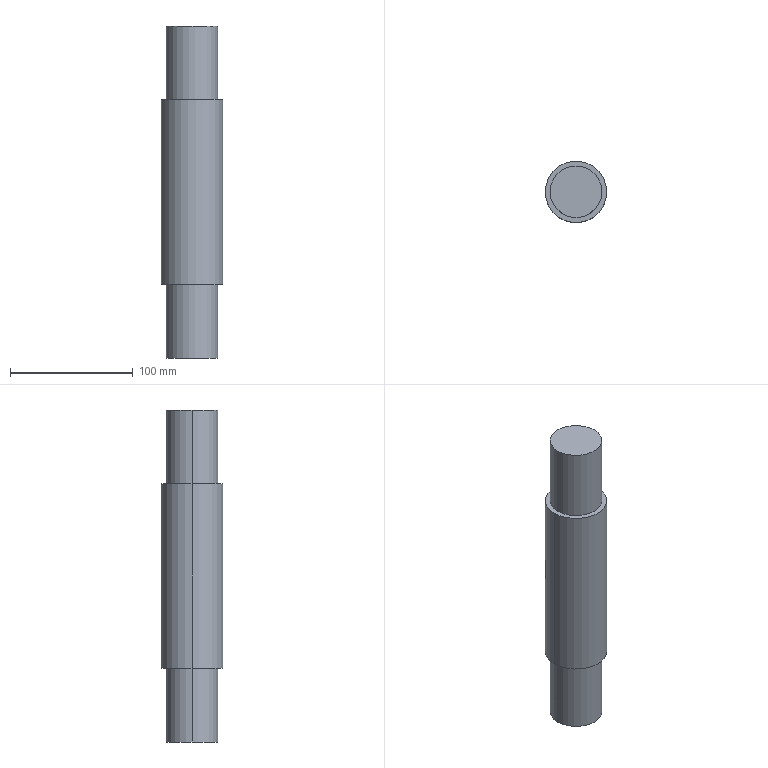Part | SolidWorks | features Extrusion 1, ICE 1, MirrorPattern 1 | 1 solid | 10 faces | box 50 x 50 x 270 mm | volume 460777 mm3 | cylinder 6 | plane 4 | commonest cylinder face diameters 42 x4 50 x2
STEP:
#1=CARTESIAN_POINT('',(21.,0.,-135.));
#2=VERTEX_POINT('',#1);
#3=CARTESIAN_POINT('',(-21.,0.,-135.));
#4=VERTEX_POINT('',#3);
#5=CARTESIAN_POINT('',(0.,0.,-135.));
#6=DIRECTION('',(0.,0.,1.));
#7=DIRECTION('',(1.,0.,0.));
#8=AXIS2_PLACEMENT_3D('',#5,#6,#7);
#9=CIRCLE('',#8,21.);
#10=EDGE_CURVE('',#2,#4,#9,.T.);
#11=ORIENTED_EDGE('',*,*,#10,.T.);
#12=CARTESIAN_POINT('',(-21.,0.,-75.));
#13=VERTEX_POINT('',#12);
#14=CARTESIAN_POINT('',(-21.,0.,-135.));
#15=DIRECTION('',(0.,0.,1.));
#16=VECTOR('',#15,1000.);
#17=LINE('',#14,#16);
#18=EDGE_CURVE('',#4,#13,#17,.T.);
#19=ORIENTED_EDGE('',*,*,#18,.T.);
#20=CARTESIAN_POINT('',(21.,0.,-75.));
#21=VERTEX_POINT('',#20);
#22=CARTESIAN_POINT('',(0.,0.,-75.));
#23=DIRECTION('',(0.,0.,1.));
#24=DIRECTION('',(1.,0.,0.));
#25=AXIS2_PLACEMENT_3D('',#22,#23,#24);
#26=CIRCLE('',#25,21.);
#27=EDGE_CURVE('',#21,#13,#26,.T.);
#28=ORIENTED_EDGE('',*,*,#27,.F.);
#29=CARTESIAN_POINT('',(21.,0.,-135.));
#30=DIRECTION('',(0.,0.,1.));
#31=VECTOR('',#30,1000.);
#32=LINE('',#29,#31);
#33=EDGE_CURVE('',#2,#21,#32,.T.);
#34=ORIENTED_EDGE('',*,*,#33,.F.);
#35=EDGE_LOOP('',(#11,#19,#28,#34));
#36=FACE_OUTER_BOUND('',#35,.T.);
#37=CARTESIAN_POINT('',(0.,0.,-135.));
#38=DIRECTION('',(0.,0.,1.));
#39=DIRECTION('',(1.,0.,0.));
#40=AXIS2_PLACEMENT_3D('',#37,#38,#39);
#41=CYLINDRICAL_SURFACE('',#40,21.);
#42=ADVANCED_FACE('',(#36),#41,.T.);
#43=CARTESIAN_POINT('',(21.,0.,135.));
#44=VERTEX_POINT('',#43);
#45=CARTESIAN_POINT('',(-21.,0.,135.));
#46=VERTEX_POINT('',#45);
#47=CARTESIAN_POINT('',(0.,0.,135.));
#48=DIRECTION('',(0.,0.,1.));
#49=DIRECTION('',(1.,0.,0.));
#50=AXIS2_PLACEMENT_3D('',#47,#48,#49);
#51=CIRCLE('',#50,21.);
#52=EDGE_CURVE('',#44,#46,#51,.T.);
#53=ORIENTED_EDGE('',*,*,#52,.F.);
#54=CARTESIAN_POINT('',(21.,0.,75.));
#55=VERTEX_POINT('',#54);
#56=CARTESIAN_POINT('',(21.,0.,135.));
#57=DIRECTION('',(0.,0.,-1.));
#58=VECTOR('',#57,1000.);
#59=LINE('',#56,#58);
#60=EDGE_CURVE('',#44,#55,#59,.T.);
#61=ORIENTED_EDGE('',*,*,#60,.T.);
#62=CARTESIAN_POINT('',(-21.,0.,75.));
#63=VERTEX_POINT('',#62);
#64=CARTESIAN_POINT('',(0.,0.,75.));
#65=DIRECTION('',(0.,0.,1.));
#66=DIRECTION('',(1.,0.,0.));
#67=AXIS2_PLACEMENT_3D('',#64,#65,#66);
#68=CIRCLE('',#67,21.);
#69=EDGE_CURVE('',#55,#63,#68,.T.);
#70=ORIENTED_EDGE('',*,*,#69,.T.);
#71=CARTESIAN_POINT('',(-21.,0.,135.));
#72=DIRECTION('',(0.,0.,-1.));
#73=VECTOR('',#72,1000.);
#74=LINE('',#71,#73);
#75=EDGE_CURVE('',#46,#63,#74,.T.);
#76=ORIENTED_EDGE('',*,*,#75,.F.);
#77=EDGE_LOOP('',(#53,#61,#70,#76));
#78=FACE_OUTER_BOUND('',#77,.T.);
#79=CARTESIAN_POINT('',(0.,0.,135.));
#80=DIRECTION('',(0.,0.,-1.));
#81=DIRECTION('',(-1.,0.,0.));
#82=AXIS2_PLACEMENT_3D('',#79,#80,#81);
#83=CYLINDRICAL_SURFACE('',#82,21.);
#84=ADVANCED_FACE('',(#78),#83,.T.);
#85=CARTESIAN_POINT('',(25.,0.,75.));
#86=VERTEX_POINT('',#85);
#87=CARTESIAN_POINT('',(-25.,0.,75.));
#88=VERTEX_POINT('',#87);
#89=CARTESIAN_POINT('',(0.,0.,75.));
#90=DIRECTION('',(0.,0.,1.));
#91=DIRECTION('',(1.,0.,0.));
#92=AXIS2_PLACEMENT_3D('',#89,#90,#91);
#93=CIRCLE('',#92,25.);
#94=EDGE_CURVE('',#86,#88,#93,.T.);
#95=ORIENTED_EDGE('',*,*,#94,.F.);
#96=CARTESIAN_POINT('',(25.,0.,-75.));
#97=VERTEX_POINT('',#96);
#98=CARTESIAN_POINT('',(25.,0.,75.));
#99=DIRECTION('',(0.,0.,-1.));
#100=VECTOR('',#99,1000.);
#101=LINE('',#98,#100);
#102=EDGE_CURVE('',#86,#97,#101,.T.);
#103=ORIENTED_EDGE('',*,*,#102,.T.);
#104=CARTESIAN_POINT('',(-25.,0.,-75.));
#105=VERTEX_POINT('',#104);
#106=CARTESIAN_POINT('',(0.,0.,-75.));
#107=DIRECTION('',(0.,0.,1.));
#108=DIRECTION('',(1.,0.,0.));
#109=AXIS2_PLACEMENT_3D('',#106,#107,#108);
#110=CIRCLE('',#109,25.);
#111=EDGE_CURVE('',#97,#105,#110,.T.);
#112=ORIENTED_EDGE('',*,*,#111,.T.);
#113=CARTESIAN_POINT('',(-25.,0.,75.));
#114=DIRECTION('',(0.,0.,-1.));
#115=VECTOR('',#114,1000.);
#116=LINE('',#113,#115);
#117=EDGE_CURVE('',#88,#105,#116,.T.);
#118=ORIENTED_EDGE('',*,*,#117,.F.);
#119=EDGE_LOOP('',(#95,#103,#112,#118));
#120=FACE_OUTER_BOUND('',#119,.T.);
#121=CARTESIAN_POINT('',(0.,0.,75.));
#122=DIRECTION('',(0.,0.,-1.));
#123=DIRECTION('',(-1.,0.,0.));
#124=AXIS2_PLACEMENT_3D('',#121,#122,#123);
#125=CYLINDRICAL_SURFACE('',#124,25.);
#126=ADVANCED_FACE('',(#120),#125,.T.);
#127=ORIENTED_EDGE('',*,*,#102,.F.);
#128=CARTESIAN_POINT('',(0.,0.,75.));
#129=DIRECTION('',(0.,0.,1.));
#130=DIRECTION('',(1.,0.,0.));
#131=AXIS2_PLACEMENT_3D('',#128,#129,#130);
#132=CIRCLE('',#131,25.);
#133=EDGE_CURVE('',#88,#86,#132,.T.);
#134=ORIENTED_EDGE('',*,*,#133,.F.);
#135=ORIENTED_EDGE('',*,*,#117,.T.);
#136=CARTESIAN_POINT('',(0.,0.,-75.));
#137=DIRECTION('',(0.,0.,1.));
#138=DIRECTION('',(1.,0.,0.));
#139=AXIS2_PLACEMENT_3D('',#136,#137,#138);
#140=CIRCLE('',#139,25.);
#141=EDGE_CURVE('',#105,#97,#140,.T.);
#142=ORIENTED_EDGE('',*,*,#141,.T.);
#143=EDGE_LOOP('',(#127,#134,#135,#142));
#144=FACE_OUTER_BOUND('',#143,.T.);
#145=CARTESIAN_POINT('',(0.,0.,75.));
#146=DIRECTION('',(0.,0.,-1.));
#147=DIRECTION('',(-1.,0.,0.));
#148=AXIS2_PLACEMENT_3D('',#145,#146,#147);
#149=CYLINDRICAL_SURFACE('',#148,25.);
#150=ADVANCED_FACE('',(#144),#149,.T.);
#151=CARTESIAN_POINT('',(0.,0.,75.));
#152=DIRECTION('',(0.,0.,1.));
#153=DIRECTION('',(1.,0.,0.));
#154=AXIS2_PLACEMENT_3D('',#151,#152,#153);
#155=CIRCLE('',#154,21.);
#156=EDGE_CURVE('',#63,#55,#155,.T.);
#157=ORIENTED_EDGE('',*,*,#156,.F.);
#158=ORIENTED_EDGE('',*,*,#69,.F.);
#159=EDGE_LOOP('',(#157,#158));
#160=FACE_BOUND('',#159,.T.);
#161=ORIENTED_EDGE('',*,*,#133,.T.);
#162=ORIENTED_EDGE('',*,*,#94,.T.);
#163=EDGE_LOOP('',(#161,#162));
#164=FACE_OUTER_BOUND('',#163,.T.);
#165=CARTESIAN_POINT('',(0.,0.,75.));
#166=DIRECTION('',(0.,0.,1.));
#167=DIRECTION('',(1.,0.,0.));
#168=AXIS2_PLACEMENT_3D('',#165,#166,#167);
#169=PLANE('',#168);
#170=ADVANCED_FACE('',(#160,#164),#169,.T.);
#171=ORIENTED_EDGE('',*,*,#27,.T.);
#172=CARTESIAN_POINT('',(0.,0.,-75.));
#173=DIRECTION('',(0.,0.,1.));
#174=DIRECTION('',(1.,0.,0.));
#175=AXIS2_PLACEMENT_3D('',#172,#173,#174);
#176=CIRCLE('',#175,21.);
#177=EDGE_CURVE('',#13,#21,#176,.T.);
#178=ORIENTED_EDGE('',*,*,#177,.T.);
#179=EDGE_LOOP('',(#171,#178));
#180=FACE_BOUND('',#179,.T.);
#181=ORIENTED_EDGE('',*,*,#141,.F.);
#182=ORIENTED_EDGE('',*,*,#111,.F.);
#183=EDGE_LOOP('',(#181,#182));
#184=FACE_OUTER_BOUND('',#183,.T.);
#185=CARTESIAN_POINT('',(0.,0.,-75.));
#186=DIRECTION('',(0.,0.,1.));
#187=DIRECTION('',(1.,0.,0.));
#188=AXIS2_PLACEMENT_3D('',#185,#186,#187);
#189=PLANE('',#188);
#190=ADVANCED_FACE('',(#180,#184),#189,.F.);
#191=ORIENTED_EDGE('',*,*,#60,.F.);
#192=CARTESIAN_POINT('',(0.,0.,135.));
#193=DIRECTION('',(0.,0.,1.));
#194=DIRECTION('',(1.,0.,0.));
#195=AXIS2_PLACEMENT_3D('',#192,#193,#194);
#196=CIRCLE('',#195,21.);
#197=EDGE_CURVE('',#46,#44,#196,.T.);
#198=ORIENTED_EDGE('',*,*,#197,.F.);
#199=ORIENTED_EDGE('',*,*,#75,.T.);
#200=ORIENTED_EDGE('',*,*,#156,.T.);
#201=EDGE_LOOP('',(#191,#198,#199,#200));
#202=FACE_OUTER_BOUND('',#201,.T.);
#203=CARTESIAN_POINT('',(0.,0.,135.));
#204=DIRECTION('',(0.,0.,-1.));
#205=DIRECTION('',(-1.,0.,0.));
#206=AXIS2_PLACEMENT_3D('',#203,#204,#205);
#207=CYLINDRICAL_SURFACE('',#206,21.);
#208=ADVANCED_FACE('',(#202),#207,.T.);
#209=ORIENTED_EDGE('',*,*,#197,.T.);
#210=ORIENTED_EDGE('',*,*,#52,.T.);
#211=EDGE_LOOP('',(#209,#210));
#212=FACE_OUTER_BOUND('',#211,.T.);
#213=CARTESIAN_POINT('',(0.,0.,135.));
#214=DIRECTION('',(0.,0.,1.));
#215=DIRECTION('',(1.,0.,0.));
#216=AXIS2_PLACEMENT_3D('',#213,#214,#215);
#217=PLANE('',#216);
#218=ADVANCED_FACE('',(#212),#217,.T.);
#219=ORIENTED_EDGE('',*,*,#18,.F.);
#220=CARTESIAN_POINT('',(0.,0.,-135.));
#221=DIRECTION('',(0.,0.,1.));
#222=DIRECTION('',(1.,0.,0.));
#223=AXIS2_PLACEMENT_3D('',#220,#221,#222);
#224=CIRCLE('',#223,21.);
#225=EDGE_CURVE('',#4,#2,#224,.T.);
#226=ORIENTED_EDGE('',*,*,#225,.T.);
#227=ORIENTED_EDGE('',*,*,#33,.T.);
#228=ORIENTED_EDGE('',*,*,#177,.F.);
#229=EDGE_LOOP('',(#219,#226,#227,#228));
#230=FACE_OUTER_BOUND('',#229,.T.);
#231=CARTESIAN_POINT('',(0.,0.,-135.));
#232=DIRECTION('',(0.,0.,1.));
#233=DIRECTION('',(1.,0.,0.));
#234=AXIS2_PLACEMENT_3D('',#231,#232,#233);
#235=CYLINDRICAL_SURFACE('',#234,21.);
#236=ADVANCED_FACE('',(#230),#235,.T.);
#237=ORIENTED_EDGE('',*,*,#10,.F.);
#238=ORIENTED_EDGE('',*,*,#225,.F.);
#239=EDGE_LOOP('',(#237,#238));
#240=FACE_OUTER_BOUND('',#239,.T.);
#241=CARTESIAN_POINT('',(0.,0.,-135.));
#242=DIRECTION('',(0.,0.,-1.));
#243=DIRECTION('',(1.,0.,0.));
#244=AXIS2_PLACEMENT_3D('',#241,#242,#243);
#245=PLANE('',#244);
#246=ADVANCED_FACE('',(#240),#245,.T.);
#247=CLOSED_SHELL('',(#42,#84,#126,#150,#170,#190,#208,#218,#236,#246));
#248=MANIFOLD_SOLID_BREP('',#247);
#249=CARTESIAN_POINT('',(0.,0.,0.));
#250=DIRECTION('',(0.,0.,1.));
#251=DIRECTION('',(1.,0.,0.));
#252=AXIS2_PLACEMENT_3D('',#249,#250,#251);
#253=(LENGTH_UNIT()NAMED_UNIT(*)SI_UNIT(.MILLI.,.METRE.));
#254=UNCERTAINTY_MEASURE_WITH_UNIT(LENGTH_MEASURE(0.00001),#253,'','');
#255=(NAMED_UNIT(*)PLANE_ANGLE_UNIT()SI_UNIT($,.RADIAN.));
#256=(NAMED_UNIT(*)SI_UNIT($,.STERADIAN.)SOLID_ANGLE_UNIT());
#257=(GEOMETRIC_REPRESENTATION_CONTEXT(3)GLOBAL_UNCERTAINTY_ASSIGNED_CONTEXT((#254))GLOBAL_UNIT_ASSIGNED_CONTEXT((#253,#255,#256))REPRESENTATION_CONTEXT('',''));
#258=ADVANCED_BREP_SHAPE_REPRESENTATION('',(#248,#252),#257);